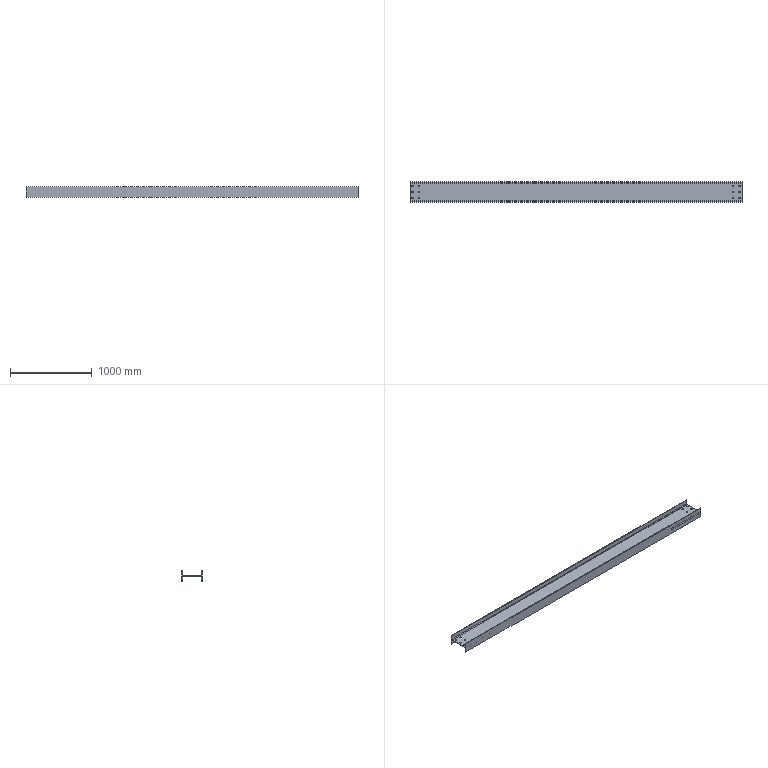Part | STEP file | 计量主梁5主体_Default<As Machined> | 1 solid | 42 faces | box 4055 x 250 x 125 mm | volume 14970670 mm3 | cylinder 28 | plane 14 | commonest cylinder face diameters 19 x24 16 x4